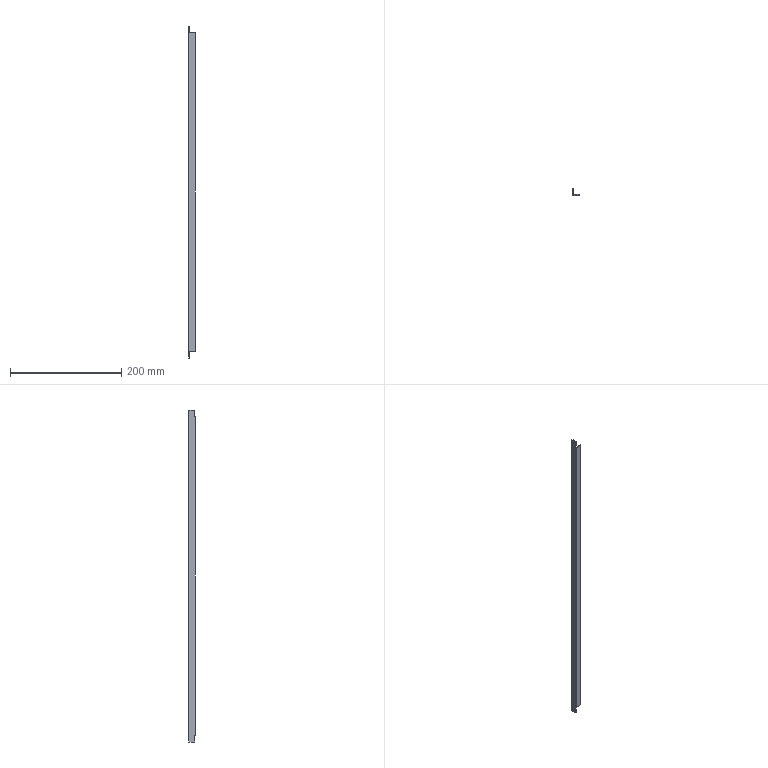Part | SolidWorks | features BaseBody 1 | 1 solid | 18 faces | box 12 x 12 x 597.2 mm | volume 15936 mm3 | plane 12 | cylinder 6 | commonest cylinder face diameters 0.6 x4 1 x2
STEP:
#1=CARTESIAN_POINT('',(0.,0.5,-286.1));
#2=VERTEX_POINT('',#1);
#3=CARTESIAN_POINT('',(0.5,0.,-286.1));
#4=VERTEX_POINT('',#3);
#5=CARTESIAN_POINT('',(0.5,0.5,-286.1));
#6=DIRECTION('',(0.,0.,1.));
#7=DIRECTION('',(-1.,0.,0.));
#8=AXIS2_PLACEMENT_3D('',#5,#6,#7);
#9=CIRCLE('',#8,0.5);
#10=EDGE_CURVE('',#2,#4,#9,.T.);
#11=ORIENTED_EDGE('',*,*,#10,.T.);
#12=CARTESIAN_POINT('',(0.5,0.,286.1));
#13=VERTEX_POINT('',#12);
#14=CARTESIAN_POINT('',(0.5,0.,0.));
#15=DIRECTION('',(0.,0.,-1.));
#16=VECTOR('',#15,1000.);
#17=LINE('',#14,#16);
#18=EDGE_CURVE('',#13,#4,#17,.T.);
#19=ORIENTED_EDGE('',*,*,#18,.F.);
#20=CARTESIAN_POINT('',(0.,0.5,286.1));
#21=VERTEX_POINT('',#20);
#22=CARTESIAN_POINT('',(0.5,0.5,286.1));
#23=DIRECTION('',(0.,0.,-1.));
#24=DIRECTION('',(-1.,0.,0.));
#25=AXIS2_PLACEMENT_3D('',#22,#23,#24);
#26=CIRCLE('',#25,0.5);
#27=EDGE_CURVE('',#13,#21,#26,.T.);
#28=ORIENTED_EDGE('',*,*,#27,.T.);
#29=CARTESIAN_POINT('',(0.,0.5,0.));
#30=DIRECTION('',(0.,0.,1.));
#31=VECTOR('',#30,1000.);
#32=LINE('',#29,#31);
#33=EDGE_CURVE('',#2,#21,#32,.T.);
#34=ORIENTED_EDGE('',*,*,#33,.F.);
#35=EDGE_LOOP('',(#11,#19,#28,#34));
#36=FACE_OUTER_BOUND('',#35,.T.);
#37=CARTESIAN_POINT('',(0.5,0.5,286.1));
#38=DIRECTION('',(0.,0.,-1.));
#39=DIRECTION('',(-1.,0.,0.));
#40=AXIS2_PLACEMENT_3D('',#37,#38,#39);
#41=CYLINDRICAL_SURFACE('',#40,0.5);
#42=ADVANCED_FACE('',(#36),#41,.T.);
#43=CARTESIAN_POINT('',(0.,1.2,-286.1));
#44=VERTEX_POINT('',#43);
#45=CARTESIAN_POINT('',(0.,1.2,-298.6));
#46=VERTEX_POINT('',#45);
#47=CARTESIAN_POINT('',(0.,1.2,0.));
#48=DIRECTION('',(0.,0.,-1.));
#49=VECTOR('',#48,1000.);
#50=LINE('',#47,#49);
#51=EDGE_CURVE('',#44,#46,#50,.T.);
#52=ORIENTED_EDGE('',*,*,#51,.F.);
#53=CARTESIAN_POINT('',(0.,0.6,-286.1));
#54=DIRECTION('',(0.,-1.,0.));
#55=VECTOR('',#54,1000.);
#56=LINE('',#53,#55);
#57=EDGE_CURVE('',#44,#2,#56,.T.);
#58=ORIENTED_EDGE('',*,*,#57,.T.);
#59=ORIENTED_EDGE('',*,*,#33,.T.);
#60=CARTESIAN_POINT('',(0.,1.2,286.1));
#61=VERTEX_POINT('',#60);
#62=CARTESIAN_POINT('',(0.,0.6,286.1));
#63=DIRECTION('',(0.,1.,0.));
#64=VECTOR('',#63,1000.);
#65=LINE('',#62,#64);
#66=EDGE_CURVE('',#21,#61,#65,.T.);
#67=ORIENTED_EDGE('',*,*,#66,.T.);
#68=CARTESIAN_POINT('',(0.,1.2,298.6));
#69=VERTEX_POINT('',#68);
#70=CARTESIAN_POINT('',(0.,1.2,0.));
#71=DIRECTION('',(0.,0.,-1.));
#72=VECTOR('',#71,1000.);
#73=LINE('',#70,#72);
#74=EDGE_CURVE('',#69,#61,#73,.T.);
#75=ORIENTED_EDGE('',*,*,#74,.F.);
#76=CARTESIAN_POINT('',(0.,11.7,298.6));
#77=VERTEX_POINT('',#76);
#78=CARTESIAN_POINT('',(0.,6.1,298.6));
#79=DIRECTION('',(0.,-1.,0.));
#80=VECTOR('',#79,1000.);
#81=LINE('',#78,#80);
#82=EDGE_CURVE('',#77,#69,#81,.T.);
#83=ORIENTED_EDGE('',*,*,#82,.F.);
#84=CARTESIAN_POINT('',(0.,11.7,-298.6));
#85=VERTEX_POINT('',#84);
#86=CARTESIAN_POINT('',(0.,11.7,0.));
#87=DIRECTION('',(0.,0.,1.));
#88=VECTOR('',#87,1000.);
#89=LINE('',#86,#88);
#90=EDGE_CURVE('',#85,#77,#89,.T.);
#91=ORIENTED_EDGE('',*,*,#90,.F.);
#92=CARTESIAN_POINT('',(0.,6.1,-298.6));
#93=DIRECTION('',(0.,1.,0.));
#94=VECTOR('',#93,1000.);
#95=LINE('',#92,#94);
#96=EDGE_CURVE('',#46,#85,#95,.T.);
#97=ORIENTED_EDGE('',*,*,#96,.F.);
#98=EDGE_LOOP('',(#52,#58,#59,#67,#75,#83,#91,#97));
#99=FACE_OUTER_BOUND('',#98,.T.);
#100=CARTESIAN_POINT('',(0.,0.5,298.6));
#101=DIRECTION('',(1.,0.,0.));
#102=DIRECTION('',(0.,0.,-1.));
#103=AXIS2_PLACEMENT_3D('',#100,#101,#102);
#104=PLANE('',#103);
#105=ADVANCED_FACE('',(#99),#104,.F.);
#106=CARTESIAN_POINT('',(11.7,0.,-286.1));
#107=VERTEX_POINT('',#106);
#108=CARTESIAN_POINT('',(6.1,0.,-286.1));
#109=DIRECTION('',(-1.,0.,0.));
#110=VECTOR('',#109,1000.);
#111=LINE('',#108,#110);
#112=EDGE_CURVE('',#107,#4,#111,.T.);
#113=ORIENTED_EDGE('',*,*,#112,.F.);
#114=CARTESIAN_POINT('',(11.7,0.,286.1));
#115=VERTEX_POINT('',#114);
#116=CARTESIAN_POINT('',(11.7,0.,0.));
#117=DIRECTION('',(0.,0.,-1.));
#118=VECTOR('',#117,1000.);
#119=LINE('',#116,#118);
#120=EDGE_CURVE('',#115,#107,#119,.T.);
#121=ORIENTED_EDGE('',*,*,#120,.F.);
#122=CARTESIAN_POINT('',(6.1,0.,286.1));
#123=DIRECTION('',(1.,0.,0.));
#124=VECTOR('',#123,1000.);
#125=LINE('',#122,#124);
#126=EDGE_CURVE('',#13,#115,#125,.T.);
#127=ORIENTED_EDGE('',*,*,#126,.F.);
#128=ORIENTED_EDGE('',*,*,#18,.T.);
#129=EDGE_LOOP('',(#113,#121,#127,#128));
#130=FACE_OUTER_BOUND('',#129,.T.);
#131=CARTESIAN_POINT('',(0.5,0.,-286.1));
#132=DIRECTION('',(0.,1.,0.));
#133=DIRECTION('',(0.,0.,1.));
#134=AXIS2_PLACEMENT_3D('',#131,#132,#133);
#135=PLANE('',#134);
#136=ADVANCED_FACE('',(#130),#135,.F.);
#137=CARTESIAN_POINT('',(1.2,11.7,-298.6));
#138=VERTEX_POINT('',#137);
#139=CARTESIAN_POINT('',(1.2,1.7,-298.6));
#140=VERTEX_POINT('',#139);
#141=CARTESIAN_POINT('',(1.2,6.6,-298.6));
#142=DIRECTION('',(0.,-1.,0.));
#143=VECTOR('',#142,1000.);
#144=LINE('',#141,#143);
#145=EDGE_CURVE('',#138,#140,#144,.T.);
#146=ORIENTED_EDGE('',*,*,#145,.T.);
#147=CARTESIAN_POINT('',(1.7,1.2,-298.6));
#148=VERTEX_POINT('',#147);
#149=CARTESIAN_POINT('',(1.7,1.7,-298.6));
#150=DIRECTION('',(0.,0.,-1.));
#151=DIRECTION('',(0.,1.,0.));
#152=AXIS2_PLACEMENT_3D('',#149,#150,#151);
#153=CIRCLE('',#152,0.5);
#154=EDGE_CURVE('',#148,#140,#153,.T.);
#155=ORIENTED_EDGE('',*,*,#154,.F.);
#156=CARTESIAN_POINT('',(0.8551,1.2,-298.6));
#157=DIRECTION('',(-1.,0.,0.));
#158=VECTOR('',#157,1000.);
#159=LINE('',#156,#158);
#160=EDGE_CURVE('',#148,#46,#159,.T.);
#161=ORIENTED_EDGE('',*,*,#160,.T.);
#162=ORIENTED_EDGE('',*,*,#96,.T.);
#163=CARTESIAN_POINT('',(0.3,12.,-298.6));
#164=VERTEX_POINT('',#163);
#165=CARTESIAN_POINT('',(0.3,11.7,-298.6));
#166=DIRECTION('',(0.,0.,-1.));
#167=DIRECTION('',(0.,1.,0.));
#168=AXIS2_PLACEMENT_3D('',#165,#166,#167);
#169=CIRCLE('',#168,0.3);
#170=EDGE_CURVE('',#85,#164,#169,.T.);
#171=ORIENTED_EDGE('',*,*,#170,.T.);
#172=CARTESIAN_POINT('',(0.9,12.,-298.6));
#173=VERTEX_POINT('',#172);
#174=CARTESIAN_POINT('',(0.6,12.,-298.6));
#175=DIRECTION('',(1.,0.,0.));
#176=VECTOR('',#175,1000.);
#177=LINE('',#174,#176);
#178=EDGE_CURVE('',#164,#173,#177,.T.);
#179=ORIENTED_EDGE('',*,*,#178,.T.);
#180=CARTESIAN_POINT('',(0.9,11.7,-298.6));
#181=DIRECTION('',(0.,0.,-1.));
#182=DIRECTION('',(0.,1.,0.));
#183=AXIS2_PLACEMENT_3D('',#180,#181,#182);
#184=CIRCLE('',#183,0.3);
#185=EDGE_CURVE('',#173,#138,#184,.T.);
#186=ORIENTED_EDGE('',*,*,#185,.T.);
#187=EDGE_LOOP('',(#146,#155,#161,#162,#171,#179,#186));
#188=FACE_OUTER_BOUND('',#187,.T.);
#189=CARTESIAN_POINT('',(1.71,1.2,-298.6));
#190=DIRECTION('',(0.,0.,-1.));
#191=DIRECTION('',(-1.,0.,0.));
#192=AXIS2_PLACEMENT_3D('',#189,#190,#191);
#193=PLANE('',#192);
#194=ADVANCED_FACE('',(#188),#193,.T.);
#195=CARTESIAN_POINT('',(1.7,1.2,-286.1));
#196=VERTEX_POINT('',#195);
#197=CARTESIAN_POINT('',(0.85,1.2,-286.1));
#198=DIRECTION('',(1.,0.,0.));
#199=VECTOR('',#198,1000.);
#200=LINE('',#197,#199);
#201=EDGE_CURVE('',#44,#196,#200,.T.);
#202=ORIENTED_EDGE('',*,*,#201,.F.);
#203=ORIENTED_EDGE('',*,*,#51,.T.);
#204=ORIENTED_EDGE('',*,*,#160,.F.);
#205=CARTESIAN_POINT('',(1.7,1.2,-292.35));
#206=DIRECTION('',(0.,0.,-1.));
#207=VECTOR('',#206,1000.);
#208=LINE('',#205,#207);
#209=EDGE_CURVE('',#196,#148,#208,.T.);
#210=ORIENTED_EDGE('',*,*,#209,.F.);
#211=EDGE_LOOP('',(#202,#203,#204,#210));
#212=FACE_OUTER_BOUND('',#211,.T.);
#213=CARTESIAN_POINT('',(0.,1.2,-298.6));
#214=DIRECTION('',(0.,1.,0.));
#215=DIRECTION('',(0.,0.,1.));
#216=AXIS2_PLACEMENT_3D('',#213,#214,#215);
#217=PLANE('',#216);
#218=ADVANCED_FACE('',(#212),#217,.F.);
#219=CARTESIAN_POINT('',(1.7,1.2,298.6));
#220=VERTEX_POINT('',#219);
#221=CARTESIAN_POINT('',(0.85,1.2,298.6));
#222=DIRECTION('',(1.,0.,0.));
#223=VECTOR('',#222,1000.);
#224=LINE('',#221,#223);
#225=EDGE_CURVE('',#69,#220,#224,.T.);
#226=ORIENTED_EDGE('',*,*,#225,.F.);
#227=ORIENTED_EDGE('',*,*,#74,.T.);
#228=CARTESIAN_POINT('',(1.7,1.2,286.1));
#229=VERTEX_POINT('',#228);
#230=CARTESIAN_POINT('',(0.85,1.2,286.1));
#231=DIRECTION('',(-1.,0.,0.));
#232=VECTOR('',#231,1000.);
#233=LINE('',#230,#232);
#234=EDGE_CURVE('',#229,#61,#233,.T.);
#235=ORIENTED_EDGE('',*,*,#234,.F.);
#236=CARTESIAN_POINT('',(1.7,1.2,292.35));
#237=DIRECTION('',(0.,0.,-1.));
#238=VECTOR('',#237,1000.);
#239=LINE('',#236,#238);
#240=EDGE_CURVE('',#220,#229,#239,.T.);
#241=ORIENTED_EDGE('',*,*,#240,.F.);
#242=EDGE_LOOP('',(#226,#227,#235,#241));
#243=FACE_OUTER_BOUND('',#242,.T.);
#244=CARTESIAN_POINT('',(0.,1.2,286.1));
#245=DIRECTION('',(0.,1.,0.));
#246=DIRECTION('',(0.,0.,1.));
#247=AXIS2_PLACEMENT_3D('',#244,#245,#246);
#248=PLANE('',#247);
#249=ADVANCED_FACE('',(#243),#248,.F.);
#250=ORIENTED_EDGE('',*,*,#225,.T.);
#251=CARTESIAN_POINT('',(1.2,1.7,298.6));
#252=VERTEX_POINT('',#251);
#253=CARTESIAN_POINT('',(1.7,1.7,298.6));
#254=DIRECTION('',(0.,0.,1.));
#255=DIRECTION('',(0.,1.,0.));
#256=AXIS2_PLACEMENT_3D('',#253,#254,#255);
#257=CIRCLE('',#256,0.5);
#258=EDGE_CURVE('',#252,#220,#257,.T.);
#259=ORIENTED_EDGE('',*,*,#258,.F.);
#260=CARTESIAN_POINT('',(1.2,11.7,298.6));
#261=VERTEX_POINT('',#260);
#262=CARTESIAN_POINT('',(1.2,6.6,298.6));
#263=DIRECTION('',(0.,-1.,0.));
#264=VECTOR('',#263,1000.);
#265=LINE('',#262,#264);
#266=EDGE_CURVE('',#261,#252,#265,.T.);
#267=ORIENTED_EDGE('',*,*,#266,.F.);
#268=CARTESIAN_POINT('',(0.9,12.,298.6));
#269=VERTEX_POINT('',#268);
#270=CARTESIAN_POINT('',(0.9,11.7,298.6));
#271=DIRECTION('',(0.,0.,1.));
#272=DIRECTION('',(0.,1.,0.));
#273=AXIS2_PLACEMENT_3D('',#270,#271,#272);
#274=CIRCLE('',#273,0.3);
#275=EDGE_CURVE('',#261,#269,#274,.T.);
#276=ORIENTED_EDGE('',*,*,#275,.T.);
#277=CARTESIAN_POINT('',(0.3,12.,298.6));
#278=VERTEX_POINT('',#277);
#279=CARTESIAN_POINT('',(0.6,12.,298.6));
#280=DIRECTION('',(-1.,0.,0.));
#281=VECTOR('',#280,1000.);
#282=LINE('',#279,#281);
#283=EDGE_CURVE('',#269,#278,#282,.T.);
#284=ORIENTED_EDGE('',*,*,#283,.T.);
#285=CARTESIAN_POINT('',(0.3,11.7,298.6));
#286=DIRECTION('',(0.,0.,-1.));
#287=DIRECTION('',(0.,1.,0.));
#288=AXIS2_PLACEMENT_3D('',#285,#286,#287);
#289=CIRCLE('',#288,0.3);
#290=EDGE_CURVE('',#77,#278,#289,.T.);
#291=ORIENTED_EDGE('',*,*,#290,.F.);
#292=ORIENTED_EDGE('',*,*,#82,.T.);
#293=EDGE_LOOP('',(#250,#259,#267,#276,#284,#291,#292));
#294=FACE_OUTER_BOUND('',#293,.T.);
#295=CARTESIAN_POINT('',(1.71,1.2,298.6));
#296=DIRECTION('',(0.,0.,-1.));
#297=DIRECTION('',(-1.,0.,0.));
#298=AXIS2_PLACEMENT_3D('',#295,#296,#297);
#299=PLANE('',#298);
#300=ADVANCED_FACE('',(#294),#299,.F.);
#301=ORIENTED_EDGE('',*,*,#90,.T.);
#302=ORIENTED_EDGE('',*,*,#290,.T.);
#303=CARTESIAN_POINT('',(0.3,12.,0.));
#304=DIRECTION('',(0.,0.,1.));
#305=VECTOR('',#304,1000.);
#306=LINE('',#303,#305);
#307=EDGE_CURVE('',#164,#278,#306,.T.);
#308=ORIENTED_EDGE('',*,*,#307,.F.);
#309=ORIENTED_EDGE('',*,*,#170,.F.);
#310=EDGE_LOOP('',(#301,#302,#308,#309));
#311=FACE_OUTER_BOUND('',#310,.T.);
#312=CARTESIAN_POINT('',(0.3,11.7,298.6));
#313=DIRECTION('',(0.,0.,-1.));
#314=DIRECTION('',(0.,1.,0.));
#315=AXIS2_PLACEMENT_3D('',#312,#313,#314);
#316=CYLINDRICAL_SURFACE('',#315,0.3);
#317=ADVANCED_FACE('',(#311),#316,.T.);
#318=ORIENTED_EDGE('',*,*,#10,.F.);
#319=ORIENTED_EDGE('',*,*,#57,.F.);
#320=ORIENTED_EDGE('',*,*,#201,.T.);
#321=CARTESIAN_POINT('',(11.7,1.2,-286.1));
#322=VERTEX_POINT('',#321);
#323=CARTESIAN_POINT('',(6.,1.2,-286.1));
#324=DIRECTION('',(-1.,0.,0.));
#325=VECTOR('',#324,1000.);
#326=LINE('',#323,#325);
#327=EDGE_CURVE('',#322,#196,#326,.T.);
#328=ORIENTED_EDGE('',*,*,#327,.F.);
#329=CARTESIAN_POINT('',(12.,0.9,-286.1));
#330=VERTEX_POINT('',#329);
#331=CARTESIAN_POINT('',(11.7,0.9,-286.1));
#332=DIRECTION('',(0.,0.,-1.));
#333=DIRECTION('',(-1.,0.,0.));
#334=AXIS2_PLACEMENT_3D('',#331,#332,#333);
#335=CIRCLE('',#334,0.3);
#336=EDGE_CURVE('',#322,#330,#335,.T.);
#337=ORIENTED_EDGE('',*,*,#336,.T.);
#338=CARTESIAN_POINT('',(12.,0.3,-286.1));
#339=VERTEX_POINT('',#338);
#340=CARTESIAN_POINT('',(12.,0.6,-286.1));
#341=DIRECTION('',(0.,-1.,0.));
#342=VECTOR('',#341,1000.);
#343=LINE('',#340,#342);
#344=EDGE_CURVE('',#330,#339,#343,.T.);
#345=ORIENTED_EDGE('',*,*,#344,.T.);
#346=CARTESIAN_POINT('',(11.7,0.3,-286.1));
#347=DIRECTION('',(0.,0.,1.));
#348=DIRECTION('',(-1.,0.,0.));
#349=AXIS2_PLACEMENT_3D('',#346,#347,#348);
#350=CIRCLE('',#349,0.3);
#351=EDGE_CURVE('',#107,#339,#350,.T.);
#352=ORIENTED_EDGE('',*,*,#351,.F.);
#353=ORIENTED_EDGE('',*,*,#112,.T.);
#354=EDGE_LOOP('',(#318,#319,#320,#328,#337,#345,#352,#353));
#355=FACE_OUTER_BOUND('',#354,.T.);
#356=CARTESIAN_POINT('',(0.,0.,-286.1));
#357=DIRECTION('',(0.,0.,1.));
#358=DIRECTION('',(1.,0.,0.));
#359=AXIS2_PLACEMENT_3D('',#356,#357,#358);
#360=PLANE('',#359);
#361=ADVANCED_FACE('',(#355),#360,.F.);
#362=ORIENTED_EDGE('',*,*,#351,.T.);
#363=CARTESIAN_POINT('',(12.,0.3,286.1));
#364=VERTEX_POINT('',#363);
#365=CARTESIAN_POINT('',(12.,0.3,0.));
#366=DIRECTION('',(0.,0.,-1.));
#367=VECTOR('',#366,1000.);
#368=LINE('',#365,#367);
#369=EDGE_CURVE('',#364,#339,#368,.T.);
#370=ORIENTED_EDGE('',*,*,#369,.F.);
#371=CARTESIAN_POINT('',(11.7,0.3,286.1));
#372=DIRECTION('',(0.,0.,1.));
#373=DIRECTION('',(-1.,0.,0.));
#374=AXIS2_PLACEMENT_3D('',#371,#372,#373);
#375=CIRCLE('',#374,0.3);
#376=EDGE_CURVE('',#115,#364,#375,.T.);
#377=ORIENTED_EDGE('',*,*,#376,.F.);
#378=ORIENTED_EDGE('',*,*,#120,.T.);
#379=EDGE_LOOP('',(#362,#370,#377,#378));
#380=FACE_OUTER_BOUND('',#379,.T.);
#381=CARTESIAN_POINT('',(11.7,0.3,286.1));
#382=DIRECTION('',(0.,0.,-1.));
#383=DIRECTION('',(-1.,0.,0.));
#384=AXIS2_PLACEMENT_3D('',#381,#382,#383);
#385=CYLINDRICAL_SURFACE('',#384,0.3);
#386=ADVANCED_FACE('',(#380),#385,.T.);
#387=CARTESIAN_POINT('',(12.,0.9,286.1));
#388=VERTEX_POINT('',#387);
#389=CARTESIAN_POINT('',(11.7,1.2,286.1));
#390=VERTEX_POINT('',#389);
#391=CARTESIAN_POINT('',(11.7,0.9,286.1));
#392=DIRECTION('',(0.,0.,1.));
#393=DIRECTION('',(-1.,0.,0.));
#394=AXIS2_PLACEMENT_3D('',#391,#392,#393);
#395=CIRCLE('',#394,0.3);
#396=EDGE_CURVE('',#388,#390,#395,.T.);
#397=ORIENTED_EDGE('',*,*,#396,.T.);
#398=CARTESIAN_POINT('',(6.,1.2,286.1));
#399=DIRECTION('',(1.,0.,0.));
#400=VECTOR('',#399,1000.);
#401=LINE('',#398,#400);
#402=EDGE_CURVE('',#229,#390,#401,.T.);
#403=ORIENTED_EDGE('',*,*,#402,.F.);
#404=ORIENTED_EDGE('',*,*,#234,.T.);
#405=ORIENTED_EDGE('',*,*,#66,.F.);
#406=ORIENTED_EDGE('',*,*,#27,.F.);
#407=ORIENTED_EDGE('',*,*,#126,.T.);
#408=ORIENTED_EDGE('',*,*,#376,.T.);
#409=CARTESIAN_POINT('',(12.,0.6,286.1));
#410=DIRECTION('',(0.,-1.,0.));
#411=VECTOR('',#410,1000.);
#412=LINE('',#409,#411);
#413=EDGE_CURVE('',#388,#364,#412,.T.);
#414=ORIENTED_EDGE('',*,*,#413,.F.);
#415=EDGE_LOOP('',(#397,#403,#404,#405,#406,#407,#408,#414));
#416=FACE_OUTER_BOUND('',#415,.T.);
#417=CARTESIAN_POINT('',(12.,0.,286.1));
#418=DIRECTION('',(0.,0.,-1.));
#419=DIRECTION('',(-1.,0.,0.));
#420=AXIS2_PLACEMENT_3D('',#417,#418,#419);
#421=PLANE('',#420);
#422=ADVANCED_FACE('',(#416),#421,.F.);
#423=CARTESIAN_POINT('',(1.2,11.7,0.));
#424=DIRECTION('',(0.,0.,-1.));
#425=VECTOR('',#424,1000.);
#426=LINE('',#423,#425);
#427=EDGE_CURVE('',#261,#138,#426,.T.);
#428=ORIENTED_EDGE('',*,*,#427,.F.);
#429=ORIENTED_EDGE('',*,*,#266,.T.);
#430=CARTESIAN_POINT('',(1.2,1.7,0.));
#431=DIRECTION('',(0.,0.,1.));
#432=VECTOR('',#431,1000.);
#433=LINE('',#430,#432);
#434=EDGE_CURVE('',#140,#252,#433,.T.);
#435=ORIENTED_EDGE('',*,*,#434,.F.);
#436=ORIENTED_EDGE('',*,*,#145,.F.);
#437=EDGE_LOOP('',(#428,#429,#435,#436));
#438=FACE_OUTER_BOUND('',#437,.T.);
#439=CARTESIAN_POINT('',(1.2,11.7,-298.6));
#440=DIRECTION('',(-1.,0.,0.));
#441=DIRECTION('',(0.,-1.,0.));
#442=AXIS2_PLACEMENT_3D('',#439,#440,#441);
#443=PLANE('',#442);
#444=ADVANCED_FACE('',(#438),#443,.F.);
#445=CARTESIAN_POINT('',(1.7,1.2,0.));
#446=DIRECTION('',(0.,0.,-1.));
#447=VECTOR('',#446,1000.);
#448=LINE('',#445,#447);
#449=EDGE_CURVE('',#229,#196,#448,.T.);
#450=ORIENTED_EDGE('',*,*,#449,.T.);
#451=ORIENTED_EDGE('',*,*,#209,.T.);
#452=ORIENTED_EDGE('',*,*,#154,.T.);
#453=ORIENTED_EDGE('',*,*,#434,.T.);
#454=ORIENTED_EDGE('',*,*,#258,.T.);
#455=ORIENTED_EDGE('',*,*,#240,.T.);
#456=EDGE_LOOP('',(#450,#451,#452,#453,#454,#455));
#457=FACE_OUTER_BOUND('',#456,.T.);
#458=CARTESIAN_POINT('',(1.7,1.7,298.6));
#459=DIRECTION('',(0.,0.,-1.));
#460=DIRECTION('',(0.,1.,0.));
#461=AXIS2_PLACEMENT_3D('',#458,#459,#460);
#462=CYLINDRICAL_SURFACE('',#461,0.5);
#463=ADVANCED_FACE('',(#457),#462,.F.);
#464=ORIENTED_EDGE('',*,*,#307,.T.);
#465=ORIENTED_EDGE('',*,*,#283,.F.);
#466=CARTESIAN_POINT('',(0.9,12.,0.));
#467=DIRECTION('',(0.,0.,1.));
#468=VECTOR('',#467,1000.);
#469=LINE('',#466,#468);
#470=EDGE_CURVE('',#173,#269,#469,.T.);
#471=ORIENTED_EDGE('',*,*,#470,.F.);
#472=ORIENTED_EDGE('',*,*,#178,.F.);
#473=EDGE_LOOP('',(#464,#465,#471,#472));
#474=FACE_OUTER_BOUND('',#473,.T.);
#475=CARTESIAN_POINT('',(0.3,12.,298.6));
#476=DIRECTION('',(0.,-1.,0.));
#477=DIRECTION('',(0.,0.,-1.));
#478=AXIS2_PLACEMENT_3D('',#475,#476,#477);
#479=PLANE('',#478);
#480=ADVANCED_FACE('',(#474),#479,.F.);
#481=ORIENTED_EDGE('',*,*,#327,.T.);
#482=ORIENTED_EDGE('',*,*,#449,.F.);
#483=ORIENTED_EDGE('',*,*,#402,.T.);
#484=CARTESIAN_POINT('',(11.7,1.2,0.));
#485=DIRECTION('',(0.,0.,1.));
#486=VECTOR('',#485,1000.);
#487=LINE('',#484,#486);
#488=EDGE_CURVE('',#322,#390,#487,.T.);
#489=ORIENTED_EDGE('',*,*,#488,.F.);
#490=EDGE_LOOP('',(#481,#482,#483,#489));
#491=FACE_OUTER_BOUND('',#490,.T.);
#492=CARTESIAN_POINT('',(1.7,1.2,-286.1));
#493=DIRECTION('',(0.,-1.,0.));
#494=DIRECTION('',(1.,0.,0.));
#495=AXIS2_PLACEMENT_3D('',#492,#493,#494);
#496=PLANE('',#495);
#497=ADVANCED_FACE('',(#491),#496,.F.);
#498=ORIENTED_EDGE('',*,*,#344,.F.);
#499=CARTESIAN_POINT('',(12.,0.9,0.));
#500=DIRECTION('',(0.,0.,-1.));
#501=VECTOR('',#500,1000.);
#502=LINE('',#499,#501);
#503=EDGE_CURVE('',#388,#330,#502,.T.);
#504=ORIENTED_EDGE('',*,*,#503,.F.);
#505=ORIENTED_EDGE('',*,*,#413,.T.);
#506=ORIENTED_EDGE('',*,*,#369,.T.);
#507=EDGE_LOOP('',(#498,#504,#505,#506));
#508=FACE_OUTER_BOUND('',#507,.T.);
#509=CARTESIAN_POINT('',(12.,0.3,-286.1));
#510=DIRECTION('',(-1.,0.,0.));
#511=DIRECTION('',(0.,0.,1.));
#512=AXIS2_PLACEMENT_3D('',#509,#510,#511);
#513=PLANE('',#512);
#514=ADVANCED_FACE('',(#508),#513,.F.);
#515=ORIENTED_EDGE('',*,*,#470,.T.);
#516=ORIENTED_EDGE('',*,*,#275,.F.);
#517=ORIENTED_EDGE('',*,*,#427,.T.);
#518=ORIENTED_EDGE('',*,*,#185,.F.);
#519=EDGE_LOOP('',(#515,#516,#517,#518));
#520=FACE_OUTER_BOUND('',#519,.T.);
#521=CARTESIAN_POINT('',(0.9,11.7,298.6));
#522=DIRECTION('',(0.,0.,-1.));
#523=DIRECTION('',(0.,1.,0.));
#524=AXIS2_PLACEMENT_3D('',#521,#522,#523);
#525=CYLINDRICAL_SURFACE('',#524,0.3);
#526=ADVANCED_FACE('',(#520),#525,.T.);
#527=ORIENTED_EDGE('',*,*,#336,.F.);
#528=ORIENTED_EDGE('',*,*,#488,.T.);
#529=ORIENTED_EDGE('',*,*,#396,.F.);
#530=ORIENTED_EDGE('',*,*,#503,.T.);
#531=EDGE_LOOP('',(#527,#528,#529,#530));
#532=FACE_OUTER_BOUND('',#531,.T.);
#533=CARTESIAN_POINT('',(11.7,0.9,286.1));
#534=DIRECTION('',(0.,0.,-1.));
#535=DIRECTION('',(-1.,0.,0.));
#536=AXIS2_PLACEMENT_3D('',#533,#534,#535);
#537=CYLINDRICAL_SURFACE('',#536,0.3);
#538=ADVANCED_FACE('',(#532),#537,.T.);
#539=CLOSED_SHELL('',(#42,#105,#136,#194,#218,#249,#300,#317,#361,#386,#422,#444,#463,#480,#497,#514,#526,#538));
#540=MANIFOLD_SOLID_BREP('',#539);
#541=CARTESIAN_POINT('',(0.,0.,0.));
#542=DIRECTION('',(0.,0.,1.));
#543=DIRECTION('',(1.,0.,0.));
#544=AXIS2_PLACEMENT_3D('',#541,#542,#543);
#545=(LENGTH_UNIT()NAMED_UNIT(*)SI_UNIT(.MILLI.,.METRE.));
#546=UNCERTAINTY_MEASURE_WITH_UNIT(LENGTH_MEASURE(0.00001),#545,'','');
#547=(NAMED_UNIT(*)PLANE_ANGLE_UNIT()SI_UNIT($,.RADIAN.));
#548=(NAMED_UNIT(*)SI_UNIT($,.STERADIAN.)SOLID_ANGLE_UNIT());
#549=(GEOMETRIC_REPRESENTATION_CONTEXT(3)GLOBAL_UNCERTAINTY_ASSIGNED_CONTEXT((#546))GLOBAL_UNIT_ASSIGNED_CONTEXT((#545,#547,#548))REPRESENTATION_CONTEXT('',''));
#550=ADVANCED_BREP_SHAPE_REPRESENTATION('',(#540,#544),#549);